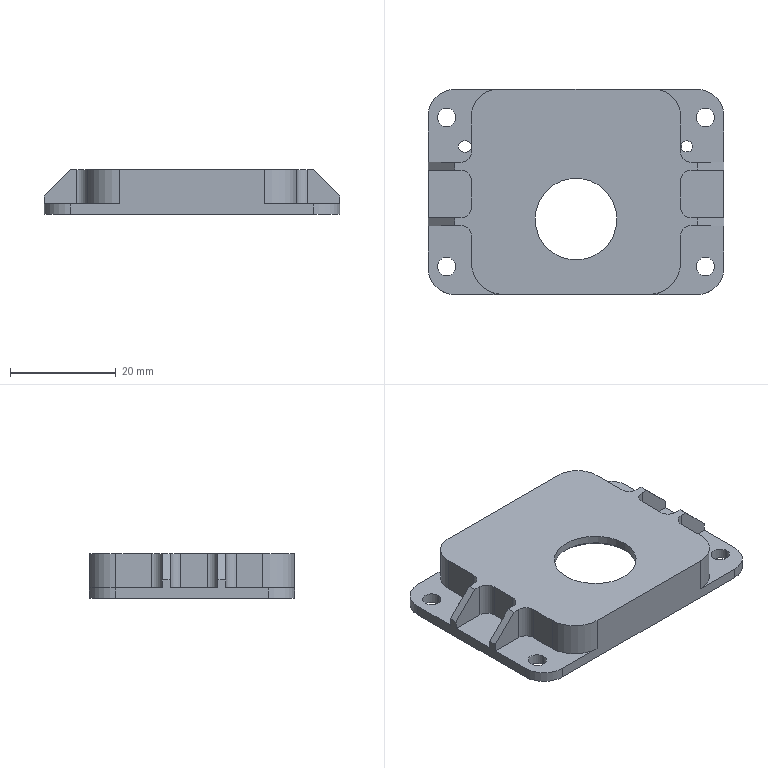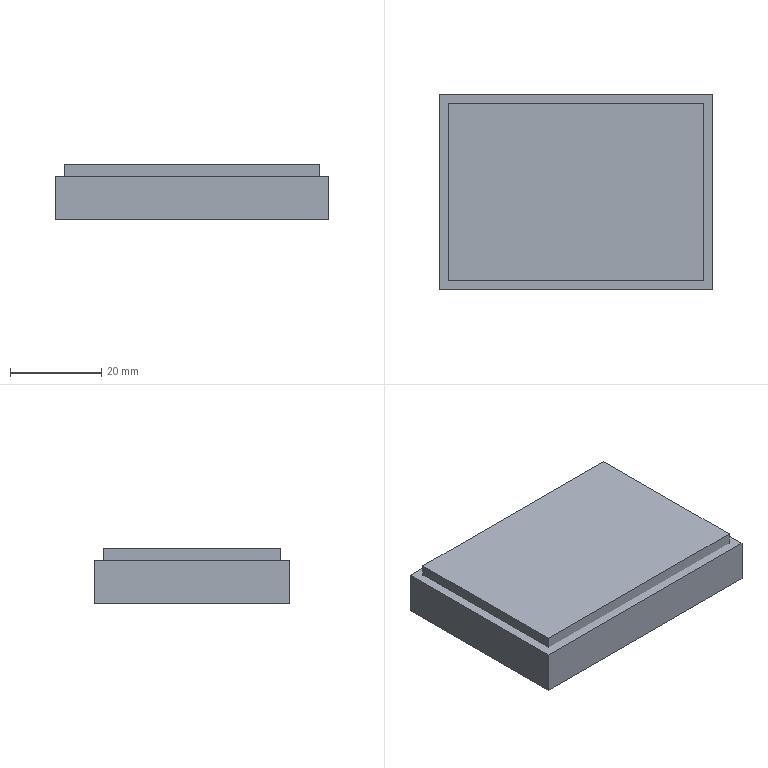CAM job | NX | 3-axis milling, drilling | part box 56 x 38.85 x 8.5 mm | stock box 60 x 42.85 x 12 mm
Tools:
number,name,description,diameter,corner_radius,flute_length,length,flutes
19,D80,Milling Tool-5 Parameters,80.0,0.0,50.0,75.0,2
15,D10,Milling Tool-5 Parameters,10.0,0.0,50.0,75.0,2
11,D4,Milling Tool-5 Parameters,4.0,0.0,50.0,75.0,2
16,D6R0.5,Milling Tool-5 Parameters,6.0,0.5,50.0,75.0,2
1,D6A45,Milling Tool-5 Parameters,6.0,0.0,50.0,75.0,2
2,2.1ZT,Drilling Tool,2.1,0.0,35.0,50.0,2
7,3.5ZT,Drilling Tool,3.5,0.0,35.0,50.0,2
20,D1.5,Milling Tool-5 Parameters,1.5,0.0,50.0,75.0,2
Operations:
program,operation,operation_type,tool,method,geometry_group,spindle_rpm,surface_speed,feed_per_tooth,feed_cut,feed_plunge,cut_length_mm,path_length_mm,cut_time_min,machine_time_min
1,FLOOR_WALL_COPY,VolumeBased25DMillingOperation,D80,METHOD,A,6500.0,1633.0,0.1154,1500.0,100.0,156.0,210.0,0.104,0.1094
1,ZLEVEL_PROFILE,ZLevelMilling,D10,METHOD,A,9500.0,298.0,0.1684,3200.0,1000.0,2020.814,2086.314,0.6636,0.6702
1,HOLE_MILLING,CylinderMilling,D10,METHOD,A,9500.0,298.0,0.1053,2000.0,100.0,66.677,128.177,0.0333,0.0395
1,CAVITY_MILL,CavityMilling,D10,METHOD,A,9500.0,298.0,0.1316,2500.0,1000.0,2310.219,2934.331,1.026,1.089
1,CAVITY_MILL_COPY,CavityMilling,D4,METHOD,A,9500.0,119.0,0.0737,1400.0,1000.0,1817.216,2974.372,1.389,1.505
1,ZLEVEL_PROFILE_COPY_1_COPY_COPY_1_COPY_COPY,ZLevelMilling,D4,METHOD,A,9500.0,298.0,0.0632,1200.0,1000.0,38.992,100.992,0.0327,0.0389
1,ZLEVEL_PROFILE_COPY_1_COPY_COPY_1_COPY_COPY_COPY,ZLevelMilling,D4,METHOD,A,9500.0,298.0,0.0632,1200.0,1000.0,196.511,271.511,0.164,0.1715
1,FLOOR_WALL,VolumeBased25DMillingOperation,D4,METHOD,A,9500.0,179.0,0.0579,1100.0,100.0,604.161,1623.983,0.5492,0.6512
1,ZLEVEL_PROFILE_1,ZLevelMilling,D6R0.5,METHOD,A,9500.0,119.0,0.1842,3500.0,100.0,841.824,1180.298,0.2405,0.2744
1,PLANAR_MILL_COPY_COPY_COPY_COPY_COPY_COPY_1_COPY_1,PlanarMilling,D6A45,METHOD,A,9500.0,179.0,0.0658,1250.0,100.0,265.074,415.443,0.2121,0.2271
1,PLANAR_MILL_COPY_COPY_COPY_COPY_COPY_COPY_1_COPY_1_COPY,PlanarMilling,D6A45,METHOD,A,9500.0,179.0,0.0658,1250.0,100.0,108.514,620.462,0.0868,0.138
2,FLOOR_WALL_COPY_COPY,VolumeBased25DMillingOperation,D80,METHOD,B,6500.0,1633.0,0.1154,1500.0,100.0,608.0,1251.501,0.4053,0.4697
2,DRILLING_COPY_1_COPY,Operation,D6A45,METHOD,B,5000.0,94.0,0.035,350.0,0.0,22.75,225.389,0.065,0.0853
2,DRILLING_COPY_1_COPY_1_1_COPY_1,Operation,2.1ZT,METHOD,B,2000.0,13.0,0.03,120.0,0.0,7.131,74.262,0.0594,0.0661
2,DRILLING_COPY_1_COPY_1_1_COPY_1_COPY,Operation,3.5ZT,METHOD,B,2000.0,13.0,0.03,120.0,0.0,30.206,235.321,0.2517,0.2722
2,CAVITY_MILL_COPY_1,CavityMilling,D10,METHOD,B,9500.0,298.0,0.1316,2500.0,1000.0,896.586,1024.575,0.3672,0.38
2,CAVITY_MILL_COPY_COPY,CavityMilling,D4,METHOD,B,9500.0,119.0,0.0737,1400.0,1000.0,2998.239,5338.938,2.265,2.499
2,FLOOR_WALL_COPY_1,VolumeBased25DMillingOperation,D4,METHOD,B,9500.0,179.0,0.0579,1100.0,100.0,1073.893,3017.607,0.9763,1.171
2,ZLEVEL_PROFILE_COPY,ZLevelMilling,D1.5,METHOD,B,9500.0,44.0,0.0526,1000.0,1000.0,71.145,132.145,0.0711,0.0772
2,PLANAR_MILL_COPY_COPY_COPY_COPY_COPY_COPY_1_COPY_1_COPY_1,PlanarMilling,D6A45,METHOD,B,9500.0,179.0,0.0658,1250.0,100.0,231.302,634.641,0.185,0.2254
2,PLANAR_MILL_COPY_COPY_COPY_COPY_COPY_COPY_1_COPY_1_COPY_1_COPY,PlanarMilling,D6A45,METHOD,B,9500.0,179.0,0.0658,1250.0,100.0,150.173,511.637,0.1201,0.1563
2,PLANAR_MILL_COPY_COPY_COPY_COPY_COPY_COPY_1_COPY_1_COPY_1_COPY_1,PlanarMilling,D6A45,METHOD,B,9500.0,179.0,0.0658,1250.0,100.0,152.908,376.942,0.1223,0.1447
2,PLANAR_MILL_COPY_COPY_COPY_COPY_COPY_COPY_1_COPY_1_COPY_1_COPY_1_COPY,PlanarMilling,D6A45,METHOD,B,9500.0,179.0,0.0658,1250.0,100.0,50.648,122.647,0.0405,0.0477